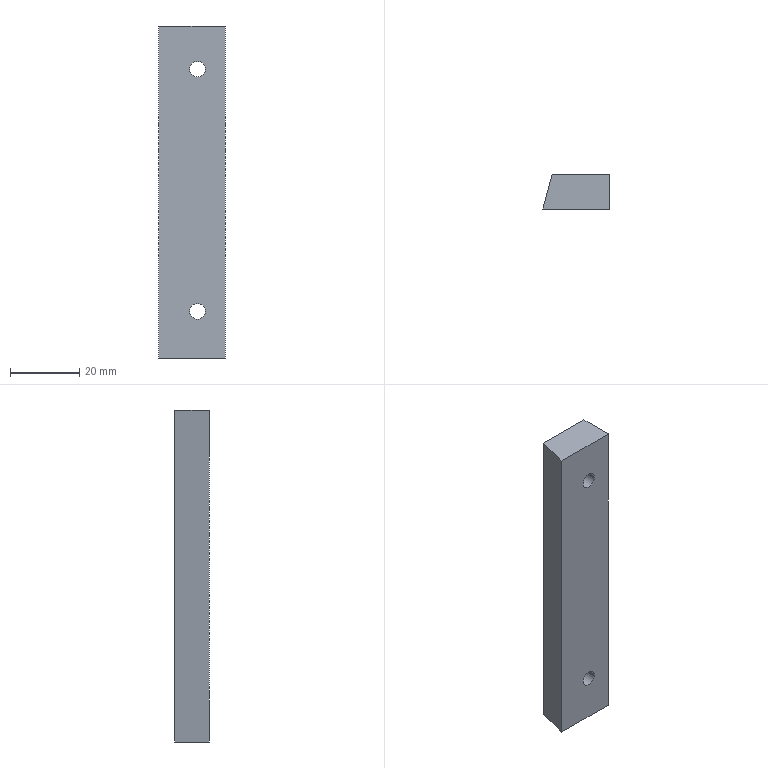Part | STEP file | X-Axis Clamp Block | 1 solid | 10 faces | box 19.179 x 10 x 96 mm | volume 16808 mm3 | plane 6 | cylinder 4 | commonest cylinder face diameters 4.5 x4
STEP:
#1=CARTESIAN_POINT('',(-1.654,-5.014,83.5));
#2=VERTEX_POINT('',#1);
#3=CARTESIAN_POINT('',(2.846,-5.014,83.5));
#4=VERTEX_POINT('',#3);
#5=CARTESIAN_POINT('',(0.5959,-5.014,83.5));
#6=DIRECTION('',(0.,-1.,0.));
#7=DIRECTION('',(-1.,0.,0.));
#8=AXIS2_PLACEMENT_3D('',#5,#6,#7);
#9=CIRCLE('',#8,2.25);
#10=EDGE_CURVE('',#2,#4,#9,.T.);
#11=ORIENTED_EDGE('',*,*,#10,.T.);
#12=CARTESIAN_POINT('',(2.846,4.986,83.5));
#13=VERTEX_POINT('',#12);
#14=CARTESIAN_POINT('',(2.846,-5.014,83.5));
#15=DIRECTION('',(0.,1.,0.));
#16=VECTOR('',#15,1000.);
#17=LINE('',#14,#16);
#18=EDGE_CURVE('',#4,#13,#17,.T.);
#19=ORIENTED_EDGE('',*,*,#18,.T.);
#20=CARTESIAN_POINT('',(-1.654,4.986,83.5));
#21=VERTEX_POINT('',#20);
#22=CARTESIAN_POINT('',(0.5959,4.986,83.5));
#23=DIRECTION('',(0.,-1.,0.));
#24=DIRECTION('',(-1.,0.,0.));
#25=AXIS2_PLACEMENT_3D('',#22,#23,#24);
#26=CIRCLE('',#25,2.25);
#27=EDGE_CURVE('',#21,#13,#26,.T.);
#28=ORIENTED_EDGE('',*,*,#27,.F.);
#29=CARTESIAN_POINT('',(-1.654,-5.014,83.5));
#30=DIRECTION('',(0.,1.,0.));
#31=VECTOR('',#30,1000.);
#32=LINE('',#29,#31);
#33=EDGE_CURVE('',#2,#21,#32,.T.);
#34=ORIENTED_EDGE('',*,*,#33,.F.);
#35=EDGE_LOOP('',(#11,#19,#28,#34));
#36=FACE_OUTER_BOUND('',#35,.T.);
#37=CARTESIAN_POINT('',(0.5959,-5.014,83.5));
#38=DIRECTION('',(0.,1.,0.));
#39=DIRECTION('',(-1.,0.,0.));
#40=AXIS2_PLACEMENT_3D('',#37,#38,#39);
#41=CYLINDRICAL_SURFACE('',#40,2.25);
#42=ADVANCED_FACE('',(#36),#41,.F.);
#43=CARTESIAN_POINT('',(-1.654,-5.014,13.5));
#44=VERTEX_POINT('',#43);
#45=CARTESIAN_POINT('',(2.846,-5.014,13.5));
#46=VERTEX_POINT('',#45);
#47=CARTESIAN_POINT('',(0.5959,-5.014,13.5));
#48=DIRECTION('',(0.,-1.,0.));
#49=DIRECTION('',(-1.,0.,0.));
#50=AXIS2_PLACEMENT_3D('',#47,#48,#49);
#51=CIRCLE('',#50,2.25);
#52=EDGE_CURVE('',#44,#46,#51,.T.);
#53=ORIENTED_EDGE('',*,*,#52,.T.);
#54=CARTESIAN_POINT('',(2.846,4.986,13.5));
#55=VERTEX_POINT('',#54);
#56=CARTESIAN_POINT('',(2.846,-5.014,13.5));
#57=DIRECTION('',(0.,1.,0.));
#58=VECTOR('',#57,1000.);
#59=LINE('',#56,#58);
#60=EDGE_CURVE('',#46,#55,#59,.T.);
#61=ORIENTED_EDGE('',*,*,#60,.T.);
#62=CARTESIAN_POINT('',(-1.654,4.986,13.5));
#63=VERTEX_POINT('',#62);
#64=CARTESIAN_POINT('',(0.5959,4.986,13.5));
#65=DIRECTION('',(0.,-1.,0.));
#66=DIRECTION('',(-1.,0.,0.));
#67=AXIS2_PLACEMENT_3D('',#64,#65,#66);
#68=CIRCLE('',#67,2.25);
#69=EDGE_CURVE('',#63,#55,#68,.T.);
#70=ORIENTED_EDGE('',*,*,#69,.F.);
#71=CARTESIAN_POINT('',(-1.654,-5.014,13.5));
#72=DIRECTION('',(0.,1.,0.));
#73=VECTOR('',#72,1000.);
#74=LINE('',#71,#73);
#75=EDGE_CURVE('',#44,#63,#74,.T.);
#76=ORIENTED_EDGE('',*,*,#75,.F.);
#77=EDGE_LOOP('',(#53,#61,#70,#76));
#78=FACE_OUTER_BOUND('',#77,.T.);
#79=CARTESIAN_POINT('',(0.5959,-5.014,13.5));
#80=DIRECTION('',(0.,1.,0.));
#81=DIRECTION('',(-1.,0.,0.));
#82=AXIS2_PLACEMENT_3D('',#79,#80,#81);
#83=CYLINDRICAL_SURFACE('',#82,2.25);
#84=ADVANCED_FACE('',(#78),#83,.F.);
#85=CARTESIAN_POINT('',(8.596,-5.014,96.));
#86=VERTEX_POINT('',#85);
#87=CARTESIAN_POINT('',(8.596,-5.014,0.));
#88=VERTEX_POINT('',#87);
#89=CARTESIAN_POINT('',(8.596,-5.014,96.));
#90=DIRECTION('',(0.,0.,-1.));
#91=VECTOR('',#90,1000.);
#92=LINE('',#89,#91);
#93=EDGE_CURVE('',#86,#88,#92,.T.);
#94=ORIENTED_EDGE('',*,*,#93,.F.);
#95=CARTESIAN_POINT('',(-10.584,-5.014,96.));
#96=VERTEX_POINT('',#95);
#97=CARTESIAN_POINT('',(8.596,-5.014,96.));
#98=DIRECTION('',(1.,0.,0.));
#99=VECTOR('',#98,1000.);
#100=LINE('',#97,#99);
#101=EDGE_CURVE('',#96,#86,#100,.T.);
#102=ORIENTED_EDGE('',*,*,#101,.F.);
#103=CARTESIAN_POINT('',(-10.584,-5.014,0.));
#104=VERTEX_POINT('',#103);
#105=CARTESIAN_POINT('',(-10.584,-5.014,96.));
#106=DIRECTION('',(0.,0.,1.));
#107=VECTOR('',#106,1000.);
#108=LINE('',#105,#107);
#109=EDGE_CURVE('',#104,#96,#108,.T.);
#110=ORIENTED_EDGE('',*,*,#109,.F.);
#111=CARTESIAN_POINT('',(8.596,-5.014,0.));
#112=DIRECTION('',(-1.,0.,0.));
#113=VECTOR('',#112,1000.);
#114=LINE('',#111,#113);
#115=EDGE_CURVE('',#88,#104,#114,.T.);
#116=ORIENTED_EDGE('',*,*,#115,.F.);
#117=EDGE_LOOP('',(#94,#102,#110,#116));
#118=FACE_OUTER_BOUND('',#117,.T.);
#119=ORIENTED_EDGE('',*,*,#10,.F.);
#120=CARTESIAN_POINT('',(0.5959,-5.014,83.5));
#121=DIRECTION('',(0.,-1.,0.));
#122=DIRECTION('',(-1.,0.,0.));
#123=AXIS2_PLACEMENT_3D('',#120,#121,#122);
#124=CIRCLE('',#123,2.25);
#125=EDGE_CURVE('',#4,#2,#124,.T.);
#126=ORIENTED_EDGE('',*,*,#125,.F.);
#127=EDGE_LOOP('',(#119,#126));
#128=FACE_BOUND('',#127,.T.);
#129=ORIENTED_EDGE('',*,*,#52,.F.);
#130=CARTESIAN_POINT('',(0.5959,-5.014,13.5));
#131=DIRECTION('',(0.,-1.,0.));
#132=DIRECTION('',(-1.,0.,0.));
#133=AXIS2_PLACEMENT_3D('',#130,#131,#132);
#134=CIRCLE('',#133,2.25);
#135=EDGE_CURVE('',#46,#44,#134,.T.);
#136=ORIENTED_EDGE('',*,*,#135,.F.);
#137=EDGE_LOOP('',(#129,#136));
#138=FACE_BOUND('',#137,.T.);
#139=CARTESIAN_POINT('',(8.596,-5.014,96.));
#140=DIRECTION('',(0.,1.,0.));
#141=DIRECTION('',(-1.,0.,0.));
#142=AXIS2_PLACEMENT_3D('',#139,#140,#141);
#143=PLANE('',#142);
#144=ADVANCED_FACE('',(#118,#128,#138),#143,.F.);
#145=ORIENTED_EDGE('',*,*,#115,.T.);
#146=CARTESIAN_POINT('',(-7.904,4.986,0.));
#147=VERTEX_POINT('',#146);
#148=CARTESIAN_POINT('',(-10.584,-5.014,0.));
#149=DIRECTION('',(0.2588,0.9659,0.));
#150=VECTOR('',#149,1000.);
#151=LINE('',#148,#150);
#152=EDGE_CURVE('',#104,#147,#151,.T.);
#153=ORIENTED_EDGE('',*,*,#152,.T.);
#154=CARTESIAN_POINT('',(8.596,4.986,0.));
#155=VERTEX_POINT('',#154);
#156=CARTESIAN_POINT('',(0.,4.986,0.));
#157=DIRECTION('',(1.,0.,0.));
#158=VECTOR('',#157,1000.);
#159=LINE('',#156,#158);
#160=EDGE_CURVE('',#147,#155,#159,.T.);
#161=ORIENTED_EDGE('',*,*,#160,.T.);
#162=CARTESIAN_POINT('',(8.596,0.,0.));
#163=DIRECTION('',(0.,-1.,0.));
#164=VECTOR('',#163,1000.);
#165=LINE('',#162,#164);
#166=EDGE_CURVE('',#155,#88,#165,.T.);
#167=ORIENTED_EDGE('',*,*,#166,.T.);
#168=EDGE_LOOP('',(#145,#153,#161,#167));
#169=FACE_OUTER_BOUND('',#168,.T.);
#170=CARTESIAN_POINT('',(0.,0.,0.));
#171=DIRECTION('',(0.,0.,-1.));
#172=DIRECTION('',(-1.,0.,0.));
#173=AXIS2_PLACEMENT_3D('',#170,#171,#172);
#174=PLANE('',#173);
#175=ADVANCED_FACE('',(#169),#174,.T.);
#176=CARTESIAN_POINT('',(8.596,4.986,96.));
#177=VERTEX_POINT('',#176);
#178=CARTESIAN_POINT('',(8.596,4.986,96.));
#179=DIRECTION('',(0.,0.,-1.));
#180=VECTOR('',#179,1000.);
#181=LINE('',#178,#180);
#182=EDGE_CURVE('',#177,#155,#181,.T.);
#183=ORIENTED_EDGE('',*,*,#182,.F.);
#184=CARTESIAN_POINT('',(8.596,4.986,96.));
#185=DIRECTION('',(0.,1.,0.));
#186=VECTOR('',#185,1000.);
#187=LINE('',#184,#186);
#188=EDGE_CURVE('',#86,#177,#187,.T.);
#189=ORIENTED_EDGE('',*,*,#188,.F.);
#190=ORIENTED_EDGE('',*,*,#93,.T.);
#191=ORIENTED_EDGE('',*,*,#166,.F.);
#192=EDGE_LOOP('',(#183,#189,#190,#191));
#193=FACE_OUTER_BOUND('',#192,.T.);
#194=CARTESIAN_POINT('',(8.596,4.986,96.));
#195=DIRECTION('',(-1.,0.,0.));
#196=DIRECTION('',(0.,-1.,0.));
#197=AXIS2_PLACEMENT_3D('',#194,#195,#196);
#198=PLANE('',#197);
#199=ADVANCED_FACE('',(#193),#198,.F.);
#200=CARTESIAN_POINT('',(-7.904,4.986,96.));
#201=VERTEX_POINT('',#200);
#202=CARTESIAN_POINT('',(-10.584,-5.014,96.));
#203=DIRECTION('',(0.2588,0.9659,0.));
#204=VECTOR('',#203,1000.);
#205=LINE('',#202,#204);
#206=EDGE_CURVE('',#96,#201,#205,.T.);
#207=ORIENTED_EDGE('',*,*,#206,.F.);
#208=ORIENTED_EDGE('',*,*,#101,.T.);
#209=ORIENTED_EDGE('',*,*,#188,.T.);
#210=CARTESIAN_POINT('',(0.,4.986,96.));
#211=DIRECTION('',(1.,0.,0.));
#212=VECTOR('',#211,1000.);
#213=LINE('',#210,#212);
#214=EDGE_CURVE('',#201,#177,#213,.T.);
#215=ORIENTED_EDGE('',*,*,#214,.F.);
#216=EDGE_LOOP('',(#207,#208,#209,#215));
#217=FACE_OUTER_BOUND('',#216,.T.);
#218=CARTESIAN_POINT('',(0.,0.,96.));
#219=DIRECTION('',(0.,0.,-1.));
#220=DIRECTION('',(-1.,0.,0.));
#221=AXIS2_PLACEMENT_3D('',#218,#219,#220);
#222=PLANE('',#221);
#223=ADVANCED_FACE('',(#217),#222,.F.);
#224=ORIENTED_EDGE('',*,*,#109,.T.);
#225=ORIENTED_EDGE('',*,*,#206,.T.);
#226=CARTESIAN_POINT('',(-7.904,4.986,96.));
#227=DIRECTION('',(0.,0.,1.));
#228=VECTOR('',#227,1000.);
#229=LINE('',#226,#228);
#230=EDGE_CURVE('',#147,#201,#229,.T.);
#231=ORIENTED_EDGE('',*,*,#230,.F.);
#232=ORIENTED_EDGE('',*,*,#152,.F.);
#233=EDGE_LOOP('',(#224,#225,#231,#232));
#234=FACE_OUTER_BOUND('',#233,.T.);
#235=CARTESIAN_POINT('',(-10.584,-5.014,96.));
#236=DIRECTION('',(0.9659,-0.2588,0.));
#237=DIRECTION('',(0.2588,0.9659,0.));
#238=AXIS2_PLACEMENT_3D('',#235,#236,#237);
#239=PLANE('',#238);
#240=ADVANCED_FACE('',(#234),#239,.F.);
#241=ORIENTED_EDGE('',*,*,#18,.F.);
#242=ORIENTED_EDGE('',*,*,#125,.T.);
#243=ORIENTED_EDGE('',*,*,#33,.T.);
#244=CARTESIAN_POINT('',(0.5959,4.986,83.5));
#245=DIRECTION('',(0.,-1.,0.));
#246=DIRECTION('',(-1.,0.,0.));
#247=AXIS2_PLACEMENT_3D('',#244,#245,#246);
#248=CIRCLE('',#247,2.25);
#249=EDGE_CURVE('',#13,#21,#248,.T.);
#250=ORIENTED_EDGE('',*,*,#249,.F.);
#251=EDGE_LOOP('',(#241,#242,#243,#250));
#252=FACE_OUTER_BOUND('',#251,.T.);
#253=CARTESIAN_POINT('',(0.5959,-5.014,83.5));
#254=DIRECTION('',(0.,1.,0.));
#255=DIRECTION('',(-1.,0.,0.));
#256=AXIS2_PLACEMENT_3D('',#253,#254,#255);
#257=CYLINDRICAL_SURFACE('',#256,2.25);
#258=ADVANCED_FACE('',(#252),#257,.F.);
#259=ORIENTED_EDGE('',*,*,#60,.F.);
#260=ORIENTED_EDGE('',*,*,#135,.T.);
#261=ORIENTED_EDGE('',*,*,#75,.T.);
#262=CARTESIAN_POINT('',(0.5959,4.986,13.5));
#263=DIRECTION('',(0.,-1.,0.));
#264=DIRECTION('',(-1.,0.,0.));
#265=AXIS2_PLACEMENT_3D('',#262,#263,#264);
#266=CIRCLE('',#265,2.25);
#267=EDGE_CURVE('',#55,#63,#266,.T.);
#268=ORIENTED_EDGE('',*,*,#267,.F.);
#269=EDGE_LOOP('',(#259,#260,#261,#268));
#270=FACE_OUTER_BOUND('',#269,.T.);
#271=CARTESIAN_POINT('',(0.5959,-5.014,13.5));
#272=DIRECTION('',(0.,1.,0.));
#273=DIRECTION('',(-1.,0.,0.));
#274=AXIS2_PLACEMENT_3D('',#271,#272,#273);
#275=CYLINDRICAL_SURFACE('',#274,2.25);
#276=ADVANCED_FACE('',(#270),#275,.F.);
#277=ORIENTED_EDGE('',*,*,#230,.T.);
#278=ORIENTED_EDGE('',*,*,#214,.T.);
#279=ORIENTED_EDGE('',*,*,#182,.T.);
#280=ORIENTED_EDGE('',*,*,#160,.F.);
#281=EDGE_LOOP('',(#277,#278,#279,#280));
#282=FACE_OUTER_BOUND('',#281,.T.);
#283=ORIENTED_EDGE('',*,*,#27,.T.);
#284=ORIENTED_EDGE('',*,*,#249,.T.);
#285=EDGE_LOOP('',(#283,#284));
#286=FACE_BOUND('',#285,.T.);
#287=ORIENTED_EDGE('',*,*,#69,.T.);
#288=ORIENTED_EDGE('',*,*,#267,.T.);
#289=EDGE_LOOP('',(#287,#288));
#290=FACE_BOUND('',#289,.T.);
#291=CARTESIAN_POINT('',(-7.904,4.986,96.));
#292=DIRECTION('',(0.,-1.,0.));
#293=DIRECTION('',(1.,0.,0.));
#294=AXIS2_PLACEMENT_3D('',#291,#292,#293);
#295=PLANE('',#294);
#296=ADVANCED_FACE('',(#282,#286,#290),#295,.F.);
#297=CLOSED_SHELL('',(#42,#84,#144,#175,#199,#223,#240,#258,#276,#296));
#298=MANIFOLD_SOLID_BREP('',#297);
#299=CARTESIAN_POINT('',(0.,0.,0.));
#300=DIRECTION('',(0.,0.,1.));
#301=DIRECTION('',(1.,0.,0.));
#302=AXIS2_PLACEMENT_3D('',#299,#300,#301);
#303=(LENGTH_UNIT()NAMED_UNIT(*)SI_UNIT(.MILLI.,.METRE.));
#304=UNCERTAINTY_MEASURE_WITH_UNIT(LENGTH_MEASURE(0.00001),#303,'','');
#305=(NAMED_UNIT(*)PLANE_ANGLE_UNIT()SI_UNIT($,.RADIAN.));
#306=(NAMED_UNIT(*)SI_UNIT($,.STERADIAN.)SOLID_ANGLE_UNIT());
#307=(GEOMETRIC_REPRESENTATION_CONTEXT(3)GLOBAL_UNCERTAINTY_ASSIGNED_CONTEXT((#304))GLOBAL_UNIT_ASSIGNED_CONTEXT((#303,#305,#306))REPRESENTATION_CONTEXT('',''));
#308=ADVANCED_BREP_SHAPE_REPRESENTATION('',(#298,#302),#307);